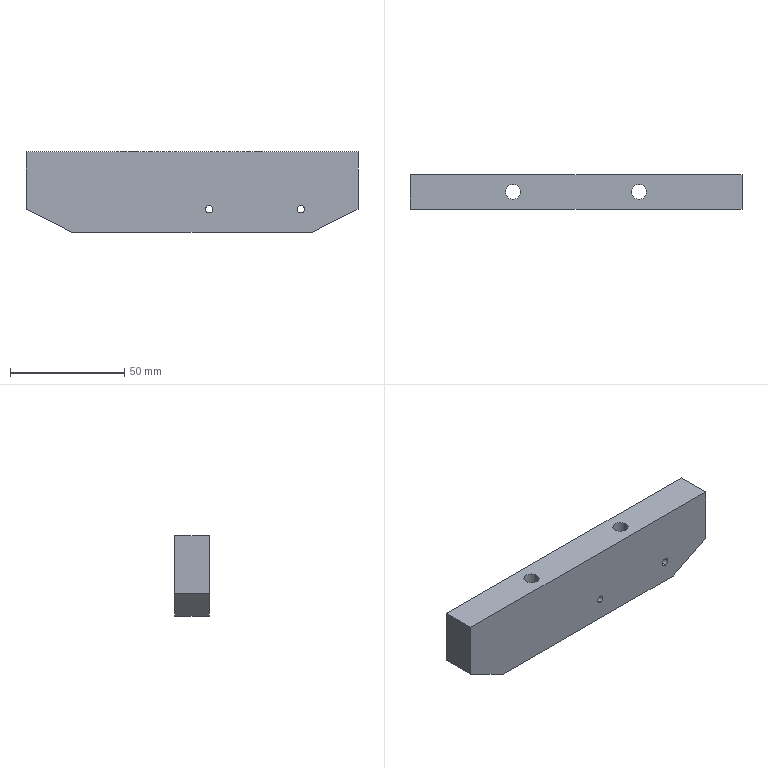Part | SolidWorks | features BaseBody 1 | 1 solid | 22 faces | box 145 x 15 x 35 mm | volume 68649 mm3 | cylinder 12 | plane 10 | commonest cylinder face diameters 3.3 x4 6.6 x4 11 x4
STEP:
#1=CARTESIAN_POINT('',(7.5,0.,-9.15));
#2=VERTEX_POINT('',#1);
#3=CARTESIAN_POINT('',(7.5,0.,-5.85));
#4=VERTEX_POINT('',#3);
#5=CARTESIAN_POINT('',(7.5,0.,-7.5));
#6=DIRECTION('',(0.,1.,0.));
#7=DIRECTION('',(0.,0.,1.));
#8=AXIS2_PLACEMENT_3D('',#5,#6,#7);
#9=CIRCLE('',#8,1.65);
#10=EDGE_CURVE('',#2,#4,#9,.T.);
#11=ORIENTED_EDGE('',*,*,#10,.F.);
#12=CARTESIAN_POINT('',(7.5,15.,-9.15));
#13=VERTEX_POINT('',#12);
#14=CARTESIAN_POINT('',(7.5,15.,-9.15));
#15=DIRECTION('',(0.,1.,0.));
#16=VECTOR('',#15,1000.);
#17=LINE('',#14,#16);
#18=EDGE_CURVE('',#2,#13,#17,.T.);
#19=ORIENTED_EDGE('',*,*,#18,.T.);
#20=CARTESIAN_POINT('',(7.5,15.,-5.85));
#21=VERTEX_POINT('',#20);
#22=CARTESIAN_POINT('',(7.5,15.,-7.5));
#23=DIRECTION('',(0.,1.,0.));
#24=DIRECTION('',(0.,0.,1.));
#25=AXIS2_PLACEMENT_3D('',#22,#23,#24);
#26=CIRCLE('',#25,1.65);
#27=EDGE_CURVE('',#13,#21,#26,.T.);
#28=ORIENTED_EDGE('',*,*,#27,.T.);
#29=CARTESIAN_POINT('',(7.5,15.,-5.85));
#30=DIRECTION('',(0.,1.,0.));
#31=VECTOR('',#30,1000.);
#32=LINE('',#29,#31);
#33=EDGE_CURVE('',#4,#21,#32,.T.);
#34=ORIENTED_EDGE('',*,*,#33,.F.);
#35=EDGE_LOOP('',(#11,#19,#28,#34));
#36=FACE_OUTER_BOUND('',#35,.T.);
#37=CARTESIAN_POINT('',(7.5,15.,-7.5));
#38=DIRECTION('',(0.,1.,0.));
#39=DIRECTION('',(0.,0.,1.));
#40=AXIS2_PLACEMENT_3D('',#37,#38,#39);
#41=CYLINDRICAL_SURFACE('',#40,1.65);
#42=ADVANCED_FACE('',(#36),#41,.F.);
#43=CARTESIAN_POINT('',(47.5,0.,-9.15));
#44=VERTEX_POINT('',#43);
#45=CARTESIAN_POINT('',(47.5,0.,-5.85));
#46=VERTEX_POINT('',#45);
#47=CARTESIAN_POINT('',(47.5,0.,-7.5));
#48=DIRECTION('',(0.,1.,0.));
#49=DIRECTION('',(0.,0.,1.));
#50=AXIS2_PLACEMENT_3D('',#47,#48,#49);
#51=CIRCLE('',#50,1.65);
#52=EDGE_CURVE('',#44,#46,#51,.T.);
#53=ORIENTED_EDGE('',*,*,#52,.F.);
#54=CARTESIAN_POINT('',(47.5,15.,-9.15));
#55=VERTEX_POINT('',#54);
#56=CARTESIAN_POINT('',(47.5,15.,-9.15));
#57=DIRECTION('',(0.,1.,0.));
#58=VECTOR('',#57,1000.);
#59=LINE('',#56,#58);
#60=EDGE_CURVE('',#44,#55,#59,.T.);
#61=ORIENTED_EDGE('',*,*,#60,.T.);
#62=CARTESIAN_POINT('',(47.5,15.,-5.85));
#63=VERTEX_POINT('',#62);
#64=CARTESIAN_POINT('',(47.5,15.,-7.5));
#65=DIRECTION('',(0.,1.,0.));
#66=DIRECTION('',(0.,0.,1.));
#67=AXIS2_PLACEMENT_3D('',#64,#65,#66);
#68=CIRCLE('',#67,1.65);
#69=EDGE_CURVE('',#55,#63,#68,.T.);
#70=ORIENTED_EDGE('',*,*,#69,.T.);
#71=CARTESIAN_POINT('',(47.5,15.,-5.85));
#72=DIRECTION('',(0.,1.,0.));
#73=VECTOR('',#72,1000.);
#74=LINE('',#71,#73);
#75=EDGE_CURVE('',#46,#63,#74,.T.);
#76=ORIENTED_EDGE('',*,*,#75,.F.);
#77=EDGE_LOOP('',(#53,#61,#70,#76));
#78=FACE_OUTER_BOUND('',#77,.T.);
#79=CARTESIAN_POINT('',(47.5,15.,-7.5));
#80=DIRECTION('',(0.,1.,0.));
#81=DIRECTION('',(0.,0.,1.));
#82=AXIS2_PLACEMENT_3D('',#79,#80,#81);
#83=CYLINDRICAL_SURFACE('',#82,1.65);
#84=ADVANCED_FACE('',(#78),#83,.F.);
#85=CARTESIAN_POINT('',(33.,7.5,-2.5));
#86=VERTEX_POINT('',#85);
#87=CARTESIAN_POINT('',(22.,7.5,-2.5));
#88=VERTEX_POINT('',#87);
#89=CARTESIAN_POINT('',(27.5,7.5,-2.5));
#90=DIRECTION('',(0.,0.,-1.));
#91=DIRECTION('',(-1.,0.,0.));
#92=AXIS2_PLACEMENT_3D('',#89,#90,#91);
#93=CIRCLE('',#92,5.5);
#94=EDGE_CURVE('',#86,#88,#93,.T.);
#95=ORIENTED_EDGE('',*,*,#94,.F.);
#96=CARTESIAN_POINT('',(33.,7.5,-17.5));
#97=VERTEX_POINT('',#96);
#98=CARTESIAN_POINT('',(33.,7.5,-17.5));
#99=DIRECTION('',(0.,0.,-1.));
#100=VECTOR('',#99,1000.);
#101=LINE('',#98,#100);
#102=EDGE_CURVE('',#86,#97,#101,.T.);
#103=ORIENTED_EDGE('',*,*,#102,.T.);
#104=CARTESIAN_POINT('',(22.,7.5,-17.5));
#105=VERTEX_POINT('',#104);
#106=CARTESIAN_POINT('',(27.5,7.5,-17.5));
#107=DIRECTION('',(0.,0.,-1.));
#108=DIRECTION('',(-1.,0.,0.));
#109=AXIS2_PLACEMENT_3D('',#106,#107,#108);
#110=CIRCLE('',#109,5.5);
#111=EDGE_CURVE('',#97,#105,#110,.T.);
#112=ORIENTED_EDGE('',*,*,#111,.T.);
#113=CARTESIAN_POINT('',(22.,7.5,-17.5));
#114=DIRECTION('',(0.,0.,-1.));
#115=VECTOR('',#114,1000.);
#116=LINE('',#113,#115);
#117=EDGE_CURVE('',#88,#105,#116,.T.);
#118=ORIENTED_EDGE('',*,*,#117,.F.);
#119=EDGE_LOOP('',(#95,#103,#112,#118));
#120=FACE_OUTER_BOUND('',#119,.T.);
#121=CARTESIAN_POINT('',(27.5,7.5,-17.5));
#122=DIRECTION('',(0.,0.,-1.));
#123=DIRECTION('',(-1.,0.,0.));
#124=AXIS2_PLACEMENT_3D('',#121,#122,#123);
#125=CYLINDRICAL_SURFACE('',#124,5.5);
#126=ADVANCED_FACE('',(#120),#125,.F.);
#127=CARTESIAN_POINT('',(30.8,7.5,17.5));
#128=VERTEX_POINT('',#127);
#129=CARTESIAN_POINT('',(24.2,7.5,17.5));
#130=VERTEX_POINT('',#129);
#131=CARTESIAN_POINT('',(27.5,7.5,17.5));
#132=DIRECTION('',(0.,0.,-1.));
#133=DIRECTION('',(-1.,0.,0.));
#134=AXIS2_PLACEMENT_3D('',#131,#132,#133);
#135=CIRCLE('',#134,3.3);
#136=EDGE_CURVE('',#128,#130,#135,.T.);
#137=ORIENTED_EDGE('',*,*,#136,.F.);
#138=CARTESIAN_POINT('',(30.8,7.5,-2.5));
#139=VERTEX_POINT('',#138);
#140=CARTESIAN_POINT('',(30.8,7.5,-17.5));
#141=DIRECTION('',(0.,0.,-1.));
#142=VECTOR('',#141,1000.);
#143=LINE('',#140,#142);
#144=EDGE_CURVE('',#128,#139,#143,.T.);
#145=ORIENTED_EDGE('',*,*,#144,.T.);
#146=CARTESIAN_POINT('',(24.2,7.5,-2.5));
#147=VERTEX_POINT('',#146);
#148=CARTESIAN_POINT('',(27.5,7.5,-2.5));
#149=DIRECTION('',(0.,0.,-1.));
#150=DIRECTION('',(-1.,0.,0.));
#151=AXIS2_PLACEMENT_3D('',#148,#149,#150);
#152=CIRCLE('',#151,3.3);
#153=EDGE_CURVE('',#139,#147,#152,.T.);
#154=ORIENTED_EDGE('',*,*,#153,.T.);
#155=CARTESIAN_POINT('',(24.2,7.5,-17.5));
#156=DIRECTION('',(0.,0.,-1.));
#157=VECTOR('',#156,1000.);
#158=LINE('',#155,#157);
#159=EDGE_CURVE('',#130,#147,#158,.T.);
#160=ORIENTED_EDGE('',*,*,#159,.F.);
#161=EDGE_LOOP('',(#137,#145,#154,#160));
#162=FACE_OUTER_BOUND('',#161,.T.);
#163=CARTESIAN_POINT('',(27.5,7.5,-17.5));
#164=DIRECTION('',(0.,0.,-1.));
#165=DIRECTION('',(-1.,0.,0.));
#166=AXIS2_PLACEMENT_3D('',#163,#164,#165);
#167=CYLINDRICAL_SURFACE('',#166,3.3);
#168=ADVANCED_FACE('',(#162),#167,.F.);
#169=CARTESIAN_POINT('',(-22.,7.5,-2.5));
#170=VERTEX_POINT('',#169);
#171=CARTESIAN_POINT('',(-33.,7.5,-2.5));
#172=VERTEX_POINT('',#171);
#173=CARTESIAN_POINT('',(-27.5,7.5,-2.5));
#174=DIRECTION('',(0.,0.,-1.));
#175=DIRECTION('',(-1.,0.,0.));
#176=AXIS2_PLACEMENT_3D('',#173,#174,#175);
#177=CIRCLE('',#176,5.5);
#178=EDGE_CURVE('',#170,#172,#177,.T.);
#179=ORIENTED_EDGE('',*,*,#178,.F.);
#180=CARTESIAN_POINT('',(-22.,7.5,-17.5));
#181=VERTEX_POINT('',#180);
#182=CARTESIAN_POINT('',(-22.,7.5,-17.5));
#183=DIRECTION('',(0.,0.,-1.));
#184=VECTOR('',#183,1000.);
#185=LINE('',#182,#184);
#186=EDGE_CURVE('',#170,#181,#185,.T.);
#187=ORIENTED_EDGE('',*,*,#186,.T.);
#188=CARTESIAN_POINT('',(-33.,7.5,-17.5));
#189=VERTEX_POINT('',#188);
#190=CARTESIAN_POINT('',(-27.5,7.5,-17.5));
#191=DIRECTION('',(0.,0.,-1.));
#192=DIRECTION('',(-1.,0.,0.));
#193=AXIS2_PLACEMENT_3D('',#190,#191,#192);
#194=CIRCLE('',#193,5.5);
#195=EDGE_CURVE('',#181,#189,#194,.T.);
#196=ORIENTED_EDGE('',*,*,#195,.T.);
#197=CARTESIAN_POINT('',(-33.,7.5,-17.5));
#198=DIRECTION('',(0.,0.,-1.));
#199=VECTOR('',#198,1000.);
#200=LINE('',#197,#199);
#201=EDGE_CURVE('',#172,#189,#200,.T.);
#202=ORIENTED_EDGE('',*,*,#201,.F.);
#203=EDGE_LOOP('',(#179,#187,#196,#202));
#204=FACE_OUTER_BOUND('',#203,.T.);
#205=CARTESIAN_POINT('',(-27.5,7.5,-17.5));
#206=DIRECTION('',(0.,0.,-1.));
#207=DIRECTION('',(-1.,0.,0.));
#208=AXIS2_PLACEMENT_3D('',#205,#206,#207);
#209=CYLINDRICAL_SURFACE('',#208,5.5);
#210=ADVANCED_FACE('',(#204),#209,.F.);
#211=CARTESIAN_POINT('',(-24.2,7.5,17.5));
#212=VERTEX_POINT('',#211);
#213=CARTESIAN_POINT('',(-30.8,7.5,17.5));
#214=VERTEX_POINT('',#213);
#215=CARTESIAN_POINT('',(-27.5,7.5,17.5));
#216=DIRECTION('',(0.,0.,-1.));
#217=DIRECTION('',(-1.,0.,0.));
#218=AXIS2_PLACEMENT_3D('',#215,#216,#217);
#219=CIRCLE('',#218,3.3);
#220=EDGE_CURVE('',#212,#214,#219,.T.);
#221=ORIENTED_EDGE('',*,*,#220,.F.);
#222=CARTESIAN_POINT('',(-24.2,7.5,-2.5));
#223=VERTEX_POINT('',#222);
#224=CARTESIAN_POINT('',(-24.2,7.5,-17.5));
#225=DIRECTION('',(0.,0.,-1.));
#226=VECTOR('',#225,1000.);
#227=LINE('',#224,#226);
#228=EDGE_CURVE('',#212,#223,#227,.T.);
#229=ORIENTED_EDGE('',*,*,#228,.T.);
#230=CARTESIAN_POINT('',(-30.8,7.5,-2.5));
#231=VERTEX_POINT('',#230);
#232=CARTESIAN_POINT('',(-27.5,7.5,-2.5));
#233=DIRECTION('',(0.,0.,-1.));
#234=DIRECTION('',(-1.,0.,0.));
#235=AXIS2_PLACEMENT_3D('',#232,#233,#234);
#236=CIRCLE('',#235,3.3);
#237=EDGE_CURVE('',#223,#231,#236,.T.);
#238=ORIENTED_EDGE('',*,*,#237,.T.);
#239=CARTESIAN_POINT('',(-30.8,7.5,-17.5));
#240=DIRECTION('',(0.,0.,-1.));
#241=VECTOR('',#240,1000.);
#242=LINE('',#239,#241);
#243=EDGE_CURVE('',#214,#231,#242,.T.);
#244=ORIENTED_EDGE('',*,*,#243,.F.);
#245=EDGE_LOOP('',(#221,#229,#238,#244));
#246=FACE_OUTER_BOUND('',#245,.T.);
#247=CARTESIAN_POINT('',(-27.5,7.5,-17.5));
#248=DIRECTION('',(0.,0.,-1.));
#249=DIRECTION('',(-1.,0.,0.));
#250=AXIS2_PLACEMENT_3D('',#247,#248,#249);
#251=CYLINDRICAL_SURFACE('',#250,3.3);
#252=ADVANCED_FACE('',(#246),#251,.F.);
#253=CARTESIAN_POINT('',(27.5,7.5,-2.5));
#254=DIRECTION('',(0.,0.,-1.));
#255=DIRECTION('',(-1.,0.,0.));
#256=AXIS2_PLACEMENT_3D('',#253,#254,#255);
#257=CIRCLE('',#256,3.3);
#258=EDGE_CURVE('',#147,#139,#257,.T.);
#259=ORIENTED_EDGE('',*,*,#258,.F.);
#260=ORIENTED_EDGE('',*,*,#153,.F.);
#261=EDGE_LOOP('',(#259,#260));
#262=FACE_BOUND('',#261,.T.);
#263=CARTESIAN_POINT('',(27.5,7.5,-2.5));
#264=DIRECTION('',(0.,0.,-1.));
#265=DIRECTION('',(-1.,0.,0.));
#266=AXIS2_PLACEMENT_3D('',#263,#264,#265);
#267=CIRCLE('',#266,5.5);
#268=EDGE_CURVE('',#88,#86,#267,.T.);
#269=ORIENTED_EDGE('',*,*,#268,.T.);
#270=ORIENTED_EDGE('',*,*,#94,.T.);
#271=EDGE_LOOP('',(#269,#270));
#272=FACE_OUTER_BOUND('',#271,.T.);
#273=CARTESIAN_POINT('',(30.8,7.5,-2.5));
#274=DIRECTION('',(0.,0.,1.));
#275=DIRECTION('',(1.,0.,0.));
#276=AXIS2_PLACEMENT_3D('',#273,#274,#275);
#277=PLANE('',#276);
#278=ADVANCED_FACE('',(#262,#272),#277,.F.);
#279=CARTESIAN_POINT('',(-27.5,7.5,-2.5));
#280=DIRECTION('',(0.,0.,-1.));
#281=DIRECTION('',(-1.,0.,0.));
#282=AXIS2_PLACEMENT_3D('',#279,#280,#281);
#283=CIRCLE('',#282,3.3);
#284=EDGE_CURVE('',#231,#223,#283,.T.);
#285=ORIENTED_EDGE('',*,*,#284,.F.);
#286=ORIENTED_EDGE('',*,*,#237,.F.);
#287=EDGE_LOOP('',(#285,#286));
#288=FACE_BOUND('',#287,.T.);
#289=CARTESIAN_POINT('',(-27.5,7.5,-2.5));
#290=DIRECTION('',(0.,0.,-1.));
#291=DIRECTION('',(-1.,0.,0.));
#292=AXIS2_PLACEMENT_3D('',#289,#290,#291);
#293=CIRCLE('',#292,5.5);
#294=EDGE_CURVE('',#172,#170,#293,.T.);
#295=ORIENTED_EDGE('',*,*,#294,.T.);
#296=ORIENTED_EDGE('',*,*,#178,.T.);
#297=EDGE_LOOP('',(#295,#296));
#298=FACE_OUTER_BOUND('',#297,.T.);
#299=CARTESIAN_POINT('',(-24.2,7.5,-2.5));
#300=DIRECTION('',(0.,0.,1.));
#301=DIRECTION('',(1.,0.,0.));
#302=AXIS2_PLACEMENT_3D('',#299,#300,#301);
#303=PLANE('',#302);
#304=ADVANCED_FACE('',(#288,#298),#303,.F.);
#305=CARTESIAN_POINT('',(72.5,15.,-7.5));
#306=VERTEX_POINT('',#305);
#307=CARTESIAN_POINT('',(52.5,15.,-17.5));
#308=VERTEX_POINT('',#307);
#309=CARTESIAN_POINT('',(17.5,15.,-35.));
#310=DIRECTION('',(-0.8944,0.,-0.4472));
#311=VECTOR('',#310,1000.);
#312=LINE('',#309,#311);
#313=EDGE_CURVE('',#306,#308,#312,.T.);
#314=ORIENTED_EDGE('',*,*,#313,.F.);
#315=CARTESIAN_POINT('',(72.5,0.,-7.5));
#316=VERTEX_POINT('',#315);
#317=CARTESIAN_POINT('',(72.5,15.,-7.5));
#318=DIRECTION('',(0.,1.,0.));
#319=VECTOR('',#318,1000.);
#320=LINE('',#317,#319);
#321=EDGE_CURVE('',#316,#306,#320,.T.);
#322=ORIENTED_EDGE('',*,*,#321,.F.);
#323=CARTESIAN_POINT('',(52.5,0.,-17.5));
#324=VERTEX_POINT('',#323);
#325=CARTESIAN_POINT('',(52.5,0.,-17.5));
#326=DIRECTION('',(0.8944,0.,0.4472));
#327=VECTOR('',#326,1000.);
#328=LINE('',#325,#327);
#329=EDGE_CURVE('',#324,#316,#328,.T.);
#330=ORIENTED_EDGE('',*,*,#329,.F.);
#331=CARTESIAN_POINT('',(52.5,15.,-17.5));
#332=DIRECTION('',(0.,-1.,0.));
#333=VECTOR('',#332,1000.);
#334=LINE('',#331,#333);
#335=EDGE_CURVE('',#308,#324,#334,.T.);
#336=ORIENTED_EDGE('',*,*,#335,.F.);
#337=EDGE_LOOP('',(#314,#322,#330,#336));
#338=FACE_OUTER_BOUND('',#337,.T.);
#339=CARTESIAN_POINT('',(52.5,15.,-17.5));
#340=DIRECTION('',(-0.4472,0.,0.8944));
#341=DIRECTION('',(0.,1.,0.));
#342=AXIS2_PLACEMENT_3D('',#339,#340,#341);
#343=PLANE('',#342);
#344=ADVANCED_FACE('',(#338),#343,.F.);
#345=CARTESIAN_POINT('',(-52.5,15.,-17.5));
#346=VERTEX_POINT('',#345);
#347=CARTESIAN_POINT('',(-72.5,15.,-7.5));
#348=VERTEX_POINT('',#347);
#349=CARTESIAN_POINT('',(-17.5,15.,-35.));
#350=DIRECTION('',(-0.8944,0.,0.4472));
#351=VECTOR('',#350,1000.);
#352=LINE('',#349,#351);
#353=EDGE_CURVE('',#346,#348,#352,.T.);
#354=ORIENTED_EDGE('',*,*,#353,.F.);
#355=CARTESIAN_POINT('',(-52.5,0.,-17.5));
#356=VERTEX_POINT('',#355);
#357=CARTESIAN_POINT('',(-52.5,15.,-17.5));
#358=DIRECTION('',(0.,1.,0.));
#359=VECTOR('',#358,1000.);
#360=LINE('',#357,#359);
#361=EDGE_CURVE('',#356,#346,#360,.T.);
#362=ORIENTED_EDGE('',*,*,#361,.F.);
#363=CARTESIAN_POINT('',(-72.5,0.,-7.5));
#364=VERTEX_POINT('',#363);
#365=CARTESIAN_POINT('',(-72.5,0.,-7.5));
#366=DIRECTION('',(0.8944,0.,-0.4472));
#367=VECTOR('',#366,1000.);
#368=LINE('',#365,#367);
#369=EDGE_CURVE('',#364,#356,#368,.T.);
#370=ORIENTED_EDGE('',*,*,#369,.F.);
#371=CARTESIAN_POINT('',(-72.5,15.,-7.5));
#372=DIRECTION('',(0.,-1.,0.));
#373=VECTOR('',#372,1000.);
#374=LINE('',#371,#373);
#375=EDGE_CURVE('',#348,#364,#374,.T.);
#376=ORIENTED_EDGE('',*,*,#375,.F.);
#377=EDGE_LOOP('',(#354,#362,#370,#376));
#378=FACE_OUTER_BOUND('',#377,.T.);
#379=CARTESIAN_POINT('',(-72.5,15.,-7.5));
#380=DIRECTION('',(0.4472,0.,0.8944));
#381=DIRECTION('',(0.,-1.,0.));
#382=AXIS2_PLACEMENT_3D('',#379,#380,#381);
#383=PLANE('',#382);
#384=ADVANCED_FACE('',(#378),#383,.F.);
#385=CARTESIAN_POINT('',(47.5,0.,-7.5));
#386=DIRECTION('',(0.,1.,0.));
#387=DIRECTION('',(0.,0.,1.));
#388=AXIS2_PLACEMENT_3D('',#385,#386,#387);
#389=CIRCLE('',#388,1.65);
#390=EDGE_CURVE('',#46,#44,#389,.T.);
#391=ORIENTED_EDGE('',*,*,#390,.T.);
#392=ORIENTED_EDGE('',*,*,#52,.T.);
#393=EDGE_LOOP('',(#391,#392));
#394=FACE_BOUND('',#393,.T.);
#395=CARTESIAN_POINT('',(7.5,0.,-7.5));
#396=DIRECTION('',(0.,1.,0.));
#397=DIRECTION('',(0.,0.,1.));
#398=AXIS2_PLACEMENT_3D('',#395,#396,#397);
#399=CIRCLE('',#398,1.65);
#400=EDGE_CURVE('',#4,#2,#399,.T.);
#401=ORIENTED_EDGE('',*,*,#400,.T.);
#402=ORIENTED_EDGE('',*,*,#10,.T.);
#403=EDGE_LOOP('',(#401,#402));
#404=FACE_BOUND('',#403,.T.);
#405=CARTESIAN_POINT('',(-72.5,0.,-17.5));
#406=DIRECTION('',(-1.,0.,0.));
#407=VECTOR('',#406,1000.);
#408=LINE('',#405,#407);
#409=EDGE_CURVE('',#324,#356,#408,.T.);
#410=ORIENTED_EDGE('',*,*,#409,.F.);
#411=ORIENTED_EDGE('',*,*,#329,.T.);
#412=CARTESIAN_POINT('',(72.5,0.,17.5));
#413=VERTEX_POINT('',#412);
#414=CARTESIAN_POINT('',(72.5,0.,-17.5));
#415=DIRECTION('',(0.,0.,-1.));
#416=VECTOR('',#415,1000.);
#417=LINE('',#414,#416);
#418=EDGE_CURVE('',#413,#316,#417,.T.);
#419=ORIENTED_EDGE('',*,*,#418,.F.);
#420=CARTESIAN_POINT('',(-72.5,0.,17.5));
#421=VERTEX_POINT('',#420);
#422=CARTESIAN_POINT('',(-72.5,0.,17.5));
#423=DIRECTION('',(1.,0.,0.));
#424=VECTOR('',#423,1000.);
#425=LINE('',#422,#424);
#426=EDGE_CURVE('',#421,#413,#425,.T.);
#427=ORIENTED_EDGE('',*,*,#426,.F.);
#428=CARTESIAN_POINT('',(-72.5,0.,-17.5));
#429=DIRECTION('',(0.,0.,1.));
#430=VECTOR('',#429,1000.);
#431=LINE('',#428,#430);
#432=EDGE_CURVE('',#364,#421,#431,.T.);
#433=ORIENTED_EDGE('',*,*,#432,.F.);
#434=ORIENTED_EDGE('',*,*,#369,.T.);
#435=EDGE_LOOP('',(#410,#411,#419,#427,#433,#434));
#436=FACE_OUTER_BOUND('',#435,.T.);
#437=CARTESIAN_POINT('',(0.,0.,0.));
#438=DIRECTION('',(0.,1.,0.));
#439=DIRECTION('',(1.,0.,0.));
#440=AXIS2_PLACEMENT_3D('',#437,#438,#439);
#441=PLANE('',#440);
#442=ADVANCED_FACE('',(#394,#404,#436),#441,.F.);
#443=CARTESIAN_POINT('',(47.5,15.,-7.5));
#444=DIRECTION('',(0.,1.,0.));
#445=DIRECTION('',(0.,0.,1.));
#446=AXIS2_PLACEMENT_3D('',#443,#444,#445);
#447=CIRCLE('',#446,1.65);
#448=EDGE_CURVE('',#63,#55,#447,.T.);
#449=ORIENTED_EDGE('',*,*,#448,.F.);
#450=ORIENTED_EDGE('',*,*,#69,.F.);
#451=EDGE_LOOP('',(#449,#450));
#452=FACE_BOUND('',#451,.T.);
#453=CARTESIAN_POINT('',(7.5,15.,-7.5));
#454=DIRECTION('',(0.,1.,0.));
#455=DIRECTION('',(0.,0.,1.));
#456=AXIS2_PLACEMENT_3D('',#453,#454,#455);
#457=CIRCLE('',#456,1.65);
#458=EDGE_CURVE('',#21,#13,#457,.T.);
#459=ORIENTED_EDGE('',*,*,#458,.F.);
#460=ORIENTED_EDGE('',*,*,#27,.F.);
#461=EDGE_LOOP('',(#459,#460));
#462=FACE_BOUND('',#461,.T.);
#463=CARTESIAN_POINT('',(72.5,15.,17.5));
#464=VERTEX_POINT('',#463);
#465=CARTESIAN_POINT('',(72.5,15.,-17.5));
#466=DIRECTION('',(0.,0.,-1.));
#467=VECTOR('',#466,1000.);
#468=LINE('',#465,#467);
#469=EDGE_CURVE('',#464,#306,#468,.T.);
#470=ORIENTED_EDGE('',*,*,#469,.T.);
#471=ORIENTED_EDGE('',*,*,#313,.T.);
#472=CARTESIAN_POINT('',(-72.5,15.,-17.5));
#473=DIRECTION('',(-1.,0.,0.));
#474=VECTOR('',#473,1000.);
#475=LINE('',#472,#474);
#476=EDGE_CURVE('',#308,#346,#475,.T.);
#477=ORIENTED_EDGE('',*,*,#476,.T.);
#478=ORIENTED_EDGE('',*,*,#353,.T.);
#479=CARTESIAN_POINT('',(-72.5,15.,17.5));
#480=VERTEX_POINT('',#479);
#481=CARTESIAN_POINT('',(-72.5,15.,-17.5));
#482=DIRECTION('',(0.,0.,1.));
#483=VECTOR('',#482,1000.);
#484=LINE('',#481,#483);
#485=EDGE_CURVE('',#348,#480,#484,.T.);
#486=ORIENTED_EDGE('',*,*,#485,.T.);
#487=CARTESIAN_POINT('',(-72.5,15.,17.5));
#488=DIRECTION('',(1.,0.,0.));
#489=VECTOR('',#488,1000.);
#490=LINE('',#487,#489);
#491=EDGE_CURVE('',#480,#464,#490,.T.);
#492=ORIENTED_EDGE('',*,*,#491,.T.);
#493=EDGE_LOOP('',(#470,#471,#477,#478,#486,#492));
#494=FACE_OUTER_BOUND('',#493,.T.);
#495=CARTESIAN_POINT('',(0.,15.,0.));
#496=DIRECTION('',(0.,1.,0.));
#497=DIRECTION('',(1.,0.,0.));
#498=AXIS2_PLACEMENT_3D('',#495,#496,#497);
#499=PLANE('',#498);
#500=ADVANCED_FACE('',(#452,#462,#494),#499,.T.);
#501=CARTESIAN_POINT('',(-27.5,7.5,17.5));
#502=DIRECTION('',(0.,0.,-1.));
#503=DIRECTION('',(-1.,0.,0.));
#504=AXIS2_PLACEMENT_3D('',#501,#502,#503);
#505=CIRCLE('',#504,3.3);
#506=EDGE_CURVE('',#214,#212,#505,.T.);
#507=ORIENTED_EDGE('',*,*,#506,.T.);
#508=ORIENTED_EDGE('',*,*,#220,.T.);
#509=EDGE_LOOP('',(#507,#508));
#510=FACE_BOUND('',#509,.T.);
#511=CARTESIAN_POINT('',(27.5,7.5,17.5));
#512=DIRECTION('',(0.,0.,-1.));
#513=DIRECTION('',(-1.,0.,0.));
#514=AXIS2_PLACEMENT_3D('',#511,#512,#513);
#515=CIRCLE('',#514,3.3);
#516=EDGE_CURVE('',#130,#128,#515,.T.);
#517=ORIENTED_EDGE('',*,*,#516,.T.);
#518=ORIENTED_EDGE('',*,*,#136,.T.);
#519=EDGE_LOOP('',(#517,#518));
#520=FACE_BOUND('',#519,.T.);
#521=ORIENTED_EDGE('',*,*,#426,.T.);
#522=CARTESIAN_POINT('',(72.5,15.,17.5));
#523=DIRECTION('',(0.,-1.,0.));
#524=VECTOR('',#523,1000.);
#525=LINE('',#522,#524);
#526=EDGE_CURVE('',#464,#413,#525,.T.);
#527=ORIENTED_EDGE('',*,*,#526,.F.);
#528=ORIENTED_EDGE('',*,*,#491,.F.);
#529=CARTESIAN_POINT('',(-72.5,15.,17.5));
#530=DIRECTION('',(0.,-1.,0.));
#531=VECTOR('',#530,1000.);
#532=LINE('',#529,#531);
#533=EDGE_CURVE('',#480,#421,#532,.T.);
#534=ORIENTED_EDGE('',*,*,#533,.T.);
#535=EDGE_LOOP('',(#521,#527,#528,#534));
#536=FACE_OUTER_BOUND('',#535,.T.);
#537=CARTESIAN_POINT('',(-72.5,15.,17.5));
#538=DIRECTION('',(0.,0.,-1.));
#539=DIRECTION('',(0.,-1.,0.));
#540=AXIS2_PLACEMENT_3D('',#537,#538,#539);
#541=PLANE('',#540);
#542=ADVANCED_FACE('',(#510,#520,#536),#541,.F.);
#543=ORIENTED_EDGE('',*,*,#485,.F.);
#544=ORIENTED_EDGE('',*,*,#375,.T.);
#545=ORIENTED_EDGE('',*,*,#432,.T.);
#546=ORIENTED_EDGE('',*,*,#533,.F.);
#547=EDGE_LOOP('',(#543,#544,#545,#546));
#548=FACE_OUTER_BOUND('',#547,.T.);
#549=CARTESIAN_POINT('',(-72.5,15.,-17.5));
#550=DIRECTION('',(1.,0.,0.));
#551=DIRECTION('',(0.,1.,0.));
#552=AXIS2_PLACEMENT_3D('',#549,#550,#551);
#553=PLANE('',#552);
#554=ADVANCED_FACE('',(#548),#553,.F.);
#555=CARTESIAN_POINT('',(-27.5,7.5,-17.5));
#556=DIRECTION('',(0.,0.,-1.));
#557=DIRECTION('',(-1.,0.,0.));
#558=AXIS2_PLACEMENT_3D('',#555,#556,#557);
#559=CIRCLE('',#558,5.5);
#560=EDGE_CURVE('',#189,#181,#559,.T.);
#561=ORIENTED_EDGE('',*,*,#560,.F.);
#562=ORIENTED_EDGE('',*,*,#195,.F.);
#563=EDGE_LOOP('',(#561,#562));
#564=FACE_BOUND('',#563,.T.);
#565=CARTESIAN_POINT('',(27.5,7.5,-17.5));
#566=DIRECTION('',(0.,0.,-1.));
#567=DIRECTION('',(-1.,0.,0.));
#568=AXIS2_PLACEMENT_3D('',#565,#566,#567);
#569=CIRCLE('',#568,5.5);
#570=EDGE_CURVE('',#105,#97,#569,.T.);
#571=ORIENTED_EDGE('',*,*,#570,.F.);
#572=ORIENTED_EDGE('',*,*,#111,.F.);
#573=EDGE_LOOP('',(#571,#572));
#574=FACE_BOUND('',#573,.T.);
#575=ORIENTED_EDGE('',*,*,#476,.F.);
#576=ORIENTED_EDGE('',*,*,#335,.T.);
#577=ORIENTED_EDGE('',*,*,#409,.T.);
#578=ORIENTED_EDGE('',*,*,#361,.T.);
#579=EDGE_LOOP('',(#575,#576,#577,#578));
#580=FACE_OUTER_BOUND('',#579,.T.);
#581=CARTESIAN_POINT('',(-72.5,15.,-17.5));
#582=DIRECTION('',(0.,0.,1.));
#583=DIRECTION('',(1.,0.,0.));
#584=AXIS2_PLACEMENT_3D('',#581,#582,#583);
#585=PLANE('',#584);
#586=ADVANCED_FACE('',(#564,#574,#580),#585,.F.);
#587=ORIENTED_EDGE('',*,*,#418,.T.);
#588=ORIENTED_EDGE('',*,*,#321,.T.);
#589=ORIENTED_EDGE('',*,*,#469,.F.);
#590=ORIENTED_EDGE('',*,*,#526,.T.);
#591=EDGE_LOOP('',(#587,#588,#589,#590));
#592=FACE_OUTER_BOUND('',#591,.T.);
#593=CARTESIAN_POINT('',(72.5,15.,-17.5));
#594=DIRECTION('',(-1.,0.,0.));
#595=DIRECTION('',(0.,0.,1.));
#596=AXIS2_PLACEMENT_3D('',#593,#594,#595);
#597=PLANE('',#596);
#598=ADVANCED_FACE('',(#592),#597,.F.);
#599=ORIENTED_EDGE('',*,*,#228,.F.);
#600=ORIENTED_EDGE('',*,*,#506,.F.);
#601=ORIENTED_EDGE('',*,*,#243,.T.);
#602=ORIENTED_EDGE('',*,*,#284,.T.);
#603=EDGE_LOOP('',(#599,#600,#601,#602));
#604=FACE_OUTER_BOUND('',#603,.T.);
#605=CARTESIAN_POINT('',(-27.5,7.5,-17.5));
#606=DIRECTION('',(0.,0.,-1.));
#607=DIRECTION('',(-1.,0.,0.));
#608=AXIS2_PLACEMENT_3D('',#605,#606,#607);
#609=CYLINDRICAL_SURFACE('',#608,3.3);
#610=ADVANCED_FACE('',(#604),#609,.F.);
#611=ORIENTED_EDGE('',*,*,#186,.F.);
#612=ORIENTED_EDGE('',*,*,#294,.F.);
#613=ORIENTED_EDGE('',*,*,#201,.T.);
#614=ORIENTED_EDGE('',*,*,#560,.T.);
#615=EDGE_LOOP('',(#611,#612,#613,#614));
#616=FACE_OUTER_BOUND('',#615,.T.);
#617=CARTESIAN_POINT('',(-27.5,7.5,-17.5));
#618=DIRECTION('',(0.,0.,-1.));
#619=DIRECTION('',(-1.,0.,0.));
#620=AXIS2_PLACEMENT_3D('',#617,#618,#619);
#621=CYLINDRICAL_SURFACE('',#620,5.5);
#622=ADVANCED_FACE('',(#616),#621,.F.);
#623=ORIENTED_EDGE('',*,*,#144,.F.);
#624=ORIENTED_EDGE('',*,*,#516,.F.);
#625=ORIENTED_EDGE('',*,*,#159,.T.);
#626=ORIENTED_EDGE('',*,*,#258,.T.);
#627=EDGE_LOOP('',(#623,#624,#625,#626));
#628=FACE_OUTER_BOUND('',#627,.T.);
#629=CARTESIAN_POINT('',(27.5,7.5,-17.5));
#630=DIRECTION('',(0.,0.,-1.));
#631=DIRECTION('',(-1.,0.,0.));
#632=AXIS2_PLACEMENT_3D('',#629,#630,#631);
#633=CYLINDRICAL_SURFACE('',#632,3.3);
#634=ADVANCED_FACE('',(#628),#633,.F.);
#635=ORIENTED_EDGE('',*,*,#102,.F.);
#636=ORIENTED_EDGE('',*,*,#268,.F.);
#637=ORIENTED_EDGE('',*,*,#117,.T.);
#638=ORIENTED_EDGE('',*,*,#570,.T.);
#639=EDGE_LOOP('',(#635,#636,#637,#638));
#640=FACE_OUTER_BOUND('',#639,.T.);
#641=CARTESIAN_POINT('',(27.5,7.5,-17.5));
#642=DIRECTION('',(0.,0.,-1.));
#643=DIRECTION('',(-1.,0.,0.));
#644=AXIS2_PLACEMENT_3D('',#641,#642,#643);
#645=CYLINDRICAL_SURFACE('',#644,5.5);
#646=ADVANCED_FACE('',(#640),#645,.F.);
#647=ORIENTED_EDGE('',*,*,#60,.F.);
#648=ORIENTED_EDGE('',*,*,#390,.F.);
#649=ORIENTED_EDGE('',*,*,#75,.T.);
#650=ORIENTED_EDGE('',*,*,#448,.T.);
#651=EDGE_LOOP('',(#647,#648,#649,#650));
#652=FACE_OUTER_BOUND('',#651,.T.);
#653=CARTESIAN_POINT('',(47.5,15.,-7.5));
#654=DIRECTION('',(0.,1.,0.));
#655=DIRECTION('',(0.,0.,1.));
#656=AXIS2_PLACEMENT_3D('',#653,#654,#655);
#657=CYLINDRICAL_SURFACE('',#656,1.65);
#658=ADVANCED_FACE('',(#652),#657,.F.);
#659=ORIENTED_EDGE('',*,*,#18,.F.);
#660=ORIENTED_EDGE('',*,*,#400,.F.);
#661=ORIENTED_EDGE('',*,*,#33,.T.);
#662=ORIENTED_EDGE('',*,*,#458,.T.);
#663=EDGE_LOOP('',(#659,#660,#661,#662));
#664=FACE_OUTER_BOUND('',#663,.T.);
#665=CARTESIAN_POINT('',(7.5,15.,-7.5));
#666=DIRECTION('',(0.,1.,0.));
#667=DIRECTION('',(0.,0.,1.));
#668=AXIS2_PLACEMENT_3D('',#665,#666,#667);
#669=CYLINDRICAL_SURFACE('',#668,1.65);
#670=ADVANCED_FACE('',(#664),#669,.F.);
#671=CLOSED_SHELL('',(#42,#84,#126,#168,#210,#252,#278,#304,#344,#384,#442,#500,#542,#554,#586,#598,#610,#622,#634,#646,#658,#670));
#672=MANIFOLD_SOLID_BREP('',#671);
#673=CARTESIAN_POINT('',(0.,0.,0.));
#674=DIRECTION('',(0.,0.,1.));
#675=DIRECTION('',(1.,0.,0.));
#676=AXIS2_PLACEMENT_3D('',#673,#674,#675);
#677=(LENGTH_UNIT()NAMED_UNIT(*)SI_UNIT(.MILLI.,.METRE.));
#678=UNCERTAINTY_MEASURE_WITH_UNIT(LENGTH_MEASURE(0.00001),#677,'','');
#679=(NAMED_UNIT(*)PLANE_ANGLE_UNIT()SI_UNIT($,.RADIAN.));
#680=(NAMED_UNIT(*)SI_UNIT($,.STERADIAN.)SOLID_ANGLE_UNIT());
#681=(GEOMETRIC_REPRESENTATION_CONTEXT(3)GLOBAL_UNCERTAINTY_ASSIGNED_CONTEXT((#678))GLOBAL_UNIT_ASSIGNED_CONTEXT((#677,#679,#680))REPRESENTATION_CONTEXT('',''));
#682=ADVANCED_BREP_SHAPE_REPRESENTATION('',(#672,#676),#681);